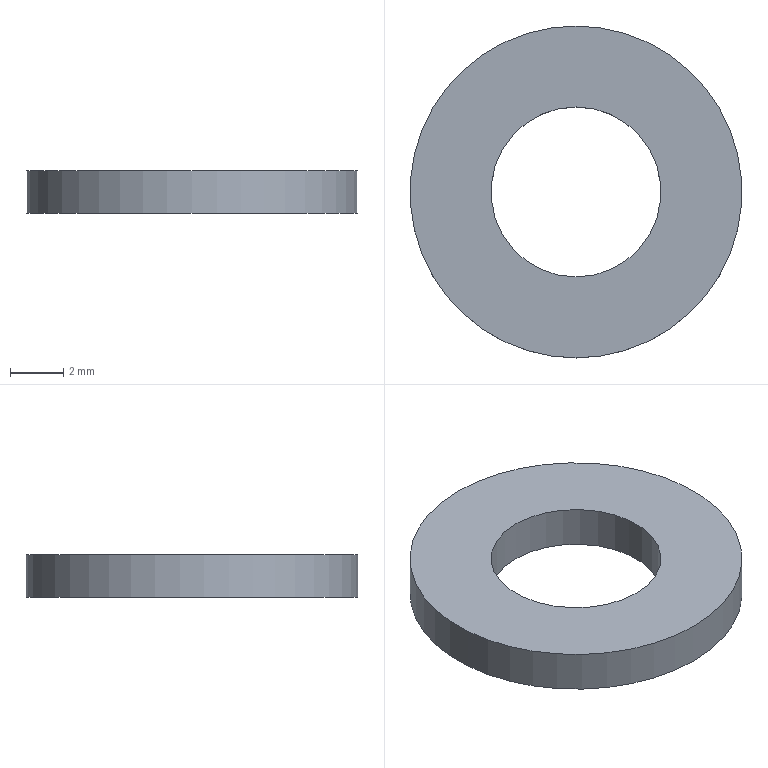Part | NX | features 5003_311_PWF6 2 | 1 solid | 4 faces | box 12.5 x 12.5 x 1.6 mm | volume 144.878 mm3 | plane 2 | cylinder 2 | commonest cylinder face diameters 6.4 x1 12.5 x1
STEP:
#1=CARTESIAN_POINT('',(141.525,-265.2,-238.));
#2=VERTEX_POINT('',#1);
#3=CARTESIAN_POINT('',(141.525,-262.,-238.));
#4=DIRECTION('',(0.,0.,-1.));
#5=DIRECTION('',(0.,-1.,0.));
#6=AXIS2_PLACEMENT_3D('',#3,#4,#5);
#7=CIRCLE('',#6,3.2);
#8=EDGE_CURVE('',#2,#2,#7,.T.);
#9=ORIENTED_EDGE('',*,*,#8,.F.);
#10=EDGE_LOOP('',(#9));
#11=FACE_BOUND('',#10,.T.);
#12=CARTESIAN_POINT('',(141.525,-268.25,-238.));
#13=VERTEX_POINT('',#12);
#14=CARTESIAN_POINT('',(141.525,-262.,-238.));
#15=DIRECTION('',(0.,0.,-1.));
#16=DIRECTION('',(0.,-1.,0.));
#17=AXIS2_PLACEMENT_3D('',#14,#15,#16);
#18=CIRCLE('',#17,6.25);
#19=EDGE_CURVE('',#13,#13,#18,.T.);
#20=ORIENTED_EDGE('',*,*,#19,.T.);
#21=EDGE_LOOP('',(#20));
#22=FACE_BOUND('',#21,.T.);
#23=CARTESIAN_POINT('',(138.325,-262.,-238.));
#24=DIRECTION('',(0.,0.,1.));
#25=DIRECTION('',(0.,1.,0.));
#26=AXIS2_PLACEMENT_3D('',#23,#24,#25);
#27=PLANE('',#26);
#28=ADVANCED_FACE('',(#11,#22),#27,.F.);
#29=ORIENTED_EDGE('',*,*,#19,.F.);
#30=EDGE_LOOP('',(#29));
#31=FACE_BOUND('',#30,.T.);
#32=CARTESIAN_POINT('',(141.525,-268.25,-236.4));
#33=VERTEX_POINT('',#32);
#34=CARTESIAN_POINT('',(141.525,-262.,-236.4));
#35=DIRECTION('',(0.,0.,-1.));
#36=DIRECTION('',(0.,-1.,0.));
#37=AXIS2_PLACEMENT_3D('',#34,#35,#36);
#38=CIRCLE('',#37,6.25);
#39=EDGE_CURVE('',#33,#33,#38,.T.);
#40=ORIENTED_EDGE('',*,*,#39,.T.);
#41=EDGE_LOOP('',(#40));
#42=FACE_BOUND('',#41,.T.);
#43=CARTESIAN_POINT('',(141.525,-262.,-238.));
#44=DIRECTION('',(0.,0.,-1.));
#45=DIRECTION('',(0.,-1.,0.));
#46=AXIS2_PLACEMENT_3D('',#43,#44,#45);
#47=CYLINDRICAL_SURFACE('',#46,6.25);
#48=ADVANCED_FACE('',(#31,#42),#47,.T.);
#49=ORIENTED_EDGE('',*,*,#39,.F.);
#50=EDGE_LOOP('',(#49));
#51=FACE_BOUND('',#50,.T.);
#52=CARTESIAN_POINT('',(141.525,-265.2,-236.4));
#53=VERTEX_POINT('',#52);
#54=CARTESIAN_POINT('',(141.525,-262.,-236.4));
#55=DIRECTION('',(0.,0.,-1.));
#56=DIRECTION('',(0.,-1.,0.));
#57=AXIS2_PLACEMENT_3D('',#54,#55,#56);
#58=CIRCLE('',#57,3.2);
#59=EDGE_CURVE('',#53,#53,#58,.T.);
#60=ORIENTED_EDGE('',*,*,#59,.T.);
#61=EDGE_LOOP('',(#60));
#62=FACE_BOUND('',#61,.T.);
#63=CARTESIAN_POINT('',(138.325,-262.,-236.4));
#64=DIRECTION('',(0.,0.,-1.));
#65=DIRECTION('',(0.,-1.,0.));
#66=AXIS2_PLACEMENT_3D('',#63,#64,#65);
#67=PLANE('',#66);
#68=ADVANCED_FACE('',(#51,#62),#67,.F.);
#69=ORIENTED_EDGE('',*,*,#59,.F.);
#70=EDGE_LOOP('',(#69));
#71=FACE_BOUND('',#70,.T.);
#72=ORIENTED_EDGE('',*,*,#8,.T.);
#73=EDGE_LOOP('',(#72));
#74=FACE_BOUND('',#73,.T.);
#75=CARTESIAN_POINT('',(141.525,-262.,-238.));
#76=DIRECTION('',(0.,0.,-1.));
#77=DIRECTION('',(0.,-1.,0.));
#78=AXIS2_PLACEMENT_3D('',#75,#76,#77);
#79=CYLINDRICAL_SURFACE('',#78,3.2);
#80=ADVANCED_FACE('',(#71,#74),#79,.F.);
#81=CLOSED_SHELL('',(#28,#48,#68,#80));
#82=MANIFOLD_SOLID_BREP('',#81);
#83=(LENGTH_UNIT()NAMED_UNIT(*)SI_UNIT(.MILLI.,.METRE.));
#84=UNCERTAINTY_MEASURE_WITH_UNIT(LENGTH_MEASURE(0.00001),#83,'','');
#85=(NAMED_UNIT(*)PLANE_ANGLE_UNIT()SI_UNIT($,.RADIAN.));
#86=(NAMED_UNIT(*)SI_UNIT($,.STERADIAN.)SOLID_ANGLE_UNIT());
#87=(GEOMETRIC_REPRESENTATION_CONTEXT(3)GLOBAL_UNCERTAINTY_ASSIGNED_CONTEXT((#84))GLOBAL_UNIT_ASSIGNED_CONTEXT((#83,#85,#86))REPRESENTATION_CONTEXT('',''));
#88=ADVANCED_BREP_SHAPE_REPRESENTATION('',(#82),#87);